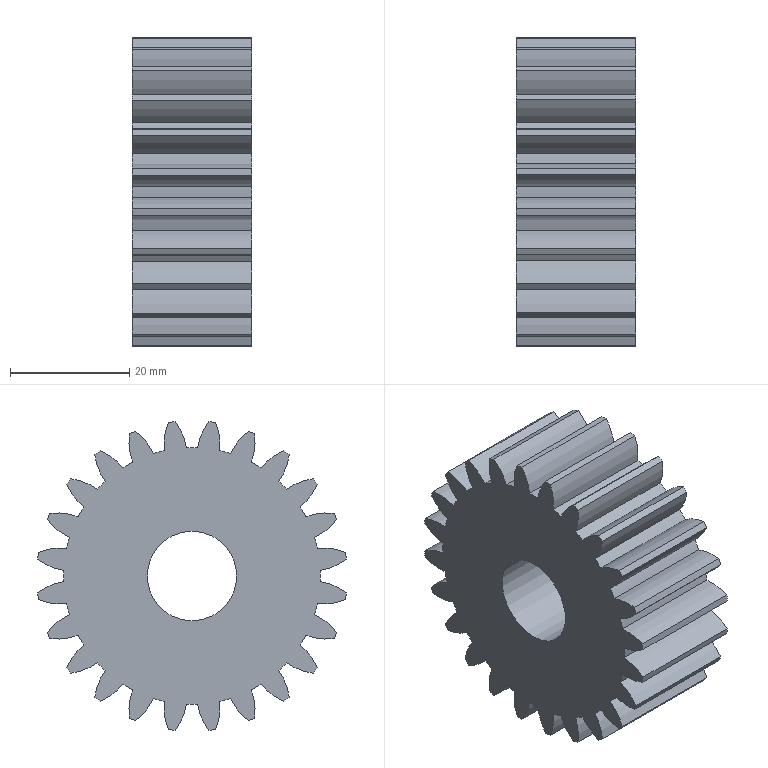Part | STEP file | spur gear_gb_GB - Spur gear 2M 24T 20PA 20FW ---S24A75H50L15.0N | 1 solid | 99 faces | box 20 x 51.691 x 51.691 mm | volume 31658 mm3 | cylinder 97 | plane 2 | commonest cylinder face diameters 19.2 x48 42.998 x24 52 x24 15 x1